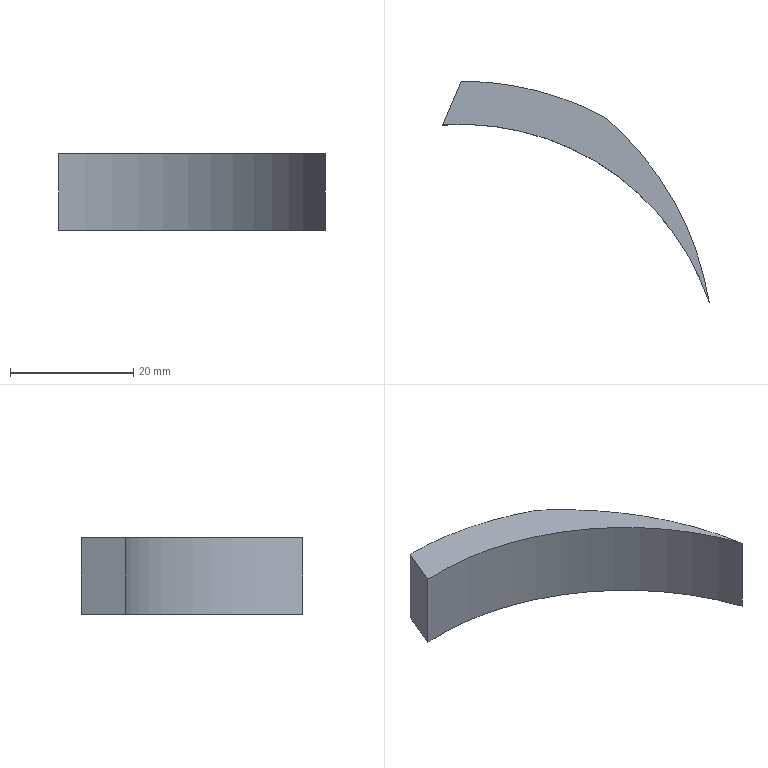Part | SolidWorks | features BaseBody 1 | 1 solid | 6 faces | box 43.285 x 35.96 x 12.5 mm | volume 3482 mm3 | cylinder 3 | plane 3 | commonest cylinder face diameters 85 x1 99 x1 100 x1
STEP:
#1=CARTESIAN_POINT('',(40.285,13.54,6.25));
#2=VERTEX_POINT('',#1);
#3=CARTESIAN_POINT('',(40.285,13.54,-6.25));
#4=VERTEX_POINT('',#3);
#5=CARTESIAN_POINT('',(40.285,13.54,6.25));
#6=DIRECTION('',(0.,0.,-1.));
#7=VECTOR('',#6,1000.);
#8=LINE('',#5,#7);
#9=EDGE_CURVE('',#2,#4,#8,.T.);
#10=ORIENTED_EDGE('',*,*,#9,.F.);
#11=CARTESIAN_POINT('',(-3.,42.394,6.25));
#12=VERTEX_POINT('',#11);
#13=CARTESIAN_POINT('',(0.,0.,6.25));
#14=DIRECTION('',(0.,0.,-1.));
#15=DIRECTION('',(-1.,0.,0.));
#16=AXIS2_PLACEMENT_3D('',#13,#14,#15);
#17=CIRCLE('',#16,42.5);
#18=EDGE_CURVE('',#12,#2,#17,.T.);
#19=ORIENTED_EDGE('',*,*,#18,.F.);
#20=CARTESIAN_POINT('',(-3.,42.394,-6.25));
#21=VERTEX_POINT('',#20);
#22=CARTESIAN_POINT('',(-3.,42.394,6.25));
#23=DIRECTION('',(0.,0.,1.));
#24=VECTOR('',#23,1000.);
#25=LINE('',#22,#24);
#26=EDGE_CURVE('',#21,#12,#25,.T.);
#27=ORIENTED_EDGE('',*,*,#26,.F.);
#28=CARTESIAN_POINT('',(0.,0.,-6.25));
#29=DIRECTION('',(0.,0.,1.));
#30=DIRECTION('',(-1.,0.,0.));
#31=AXIS2_PLACEMENT_3D('',#28,#29,#30);
#32=CIRCLE('',#31,42.5);
#33=EDGE_CURVE('',#4,#21,#32,.T.);
#34=ORIENTED_EDGE('',*,*,#33,.F.);
#35=EDGE_LOOP('',(#10,#19,#27,#34));
#36=FACE_OUTER_BOUND('',#35,.T.);
#37=CARTESIAN_POINT('',(0.,0.,6.25));
#38=DIRECTION('',(0.,0.,-1.));
#39=DIRECTION('',(-1.,0.,0.));
#40=AXIS2_PLACEMENT_3D('',#37,#38,#39);
#41=CYLINDRICAL_SURFACE('',#40,42.5);
#42=ADVANCED_FACE('',(#36),#41,.F.);
#43=CARTESIAN_POINT('',(23.284,43.682,-6.25));
#44=VERTEX_POINT('',#43);
#45=CARTESIAN_POINT('',(-9.074,5.565,-6.25));
#46=DIRECTION('',(0.,0.,1.));
#47=DIRECTION('',(-1.,0.,0.));
#48=AXIS2_PLACEMENT_3D('',#45,#46,#47);
#49=CIRCLE('',#48,50.);
#50=EDGE_CURVE('',#4,#44,#49,.T.);
#51=ORIENTED_EDGE('',*,*,#50,.F.);
#52=ORIENTED_EDGE('',*,*,#33,.T.);
#53=CARTESIAN_POINT('',(0.,49.5,-6.25));
#54=VERTEX_POINT('',#53);
#55=CARTESIAN_POINT('',(0.,49.5,-6.25));
#56=DIRECTION('',(-0.3889,-0.9213,0.));
#57=VECTOR('',#56,1000.);
#58=LINE('',#55,#57);
#59=EDGE_CURVE('',#54,#21,#58,.T.);
#60=ORIENTED_EDGE('',*,*,#59,.F.);
#61=CARTESIAN_POINT('',(0.,0.,-6.25));
#62=DIRECTION('',(0.,0.,1.));
#63=DIRECTION('',(-1.,0.,0.));
#64=AXIS2_PLACEMENT_3D('',#61,#62,#63);
#65=CIRCLE('',#64,49.5);
#66=EDGE_CURVE('',#44,#54,#65,.T.);
#67=ORIENTED_EDGE('',*,*,#66,.F.);
#68=EDGE_LOOP('',(#51,#52,#60,#67));
#69=FACE_OUTER_BOUND('',#68,.T.);
#70=CARTESIAN_POINT('',(0.,0.,-6.25));
#71=DIRECTION('',(0.,0.,1.));
#72=DIRECTION('',(1.,0.,0.));
#73=AXIS2_PLACEMENT_3D('',#70,#71,#72);
#74=PLANE('',#73);
#75=ADVANCED_FACE('',(#69),#74,.F.);
#76=CARTESIAN_POINT('',(23.284,43.682,6.25));
#77=VERTEX_POINT('',#76);
#78=CARTESIAN_POINT('',(-9.074,5.565,6.25));
#79=DIRECTION('',(0.,0.,-1.));
#80=DIRECTION('',(-1.,0.,0.));
#81=AXIS2_PLACEMENT_3D('',#78,#79,#80);
#82=CIRCLE('',#81,50.);
#83=EDGE_CURVE('',#77,#2,#82,.T.);
#84=ORIENTED_EDGE('',*,*,#83,.T.);
#85=ORIENTED_EDGE('',*,*,#9,.T.);
#86=ORIENTED_EDGE('',*,*,#50,.T.);
#87=CARTESIAN_POINT('',(23.284,43.682,6.25));
#88=DIRECTION('',(0.,0.,1.));
#89=VECTOR('',#88,1000.);
#90=LINE('',#87,#89);
#91=EDGE_CURVE('',#44,#77,#90,.T.);
#92=ORIENTED_EDGE('',*,*,#91,.T.);
#93=EDGE_LOOP('',(#84,#85,#86,#92));
#94=FACE_OUTER_BOUND('',#93,.T.);
#95=CARTESIAN_POINT('',(-9.074,5.565,6.25));
#96=DIRECTION('',(0.,0.,-1.));
#97=DIRECTION('',(-1.,0.,0.));
#98=AXIS2_PLACEMENT_3D('',#95,#96,#97);
#99=CYLINDRICAL_SURFACE('',#98,50.);
#100=ADVANCED_FACE('',(#94),#99,.T.);
#101=ORIENTED_EDGE('',*,*,#18,.T.);
#102=ORIENTED_EDGE('',*,*,#83,.F.);
#103=CARTESIAN_POINT('',(0.,49.5,6.25));
#104=VERTEX_POINT('',#103);
#105=CARTESIAN_POINT('',(0.,0.,6.25));
#106=DIRECTION('',(0.,0.,1.));
#107=DIRECTION('',(-1.,0.,0.));
#108=AXIS2_PLACEMENT_3D('',#105,#106,#107);
#109=CIRCLE('',#108,49.5);
#110=EDGE_CURVE('',#77,#104,#109,.T.);
#111=ORIENTED_EDGE('',*,*,#110,.T.);
#112=CARTESIAN_POINT('',(0.,49.5,6.25));
#113=DIRECTION('',(-0.3889,-0.9213,0.));
#114=VECTOR('',#113,1000.);
#115=LINE('',#112,#114);
#116=EDGE_CURVE('',#104,#12,#115,.T.);
#117=ORIENTED_EDGE('',*,*,#116,.T.);
#118=EDGE_LOOP('',(#101,#102,#111,#117));
#119=FACE_OUTER_BOUND('',#118,.T.);
#120=CARTESIAN_POINT('',(0.,0.,6.25));
#121=DIRECTION('',(0.,0.,1.));
#122=DIRECTION('',(1.,0.,0.));
#123=AXIS2_PLACEMENT_3D('',#120,#121,#122);
#124=PLANE('',#123);
#125=ADVANCED_FACE('',(#119),#124,.T.);
#126=ORIENTED_EDGE('',*,*,#26,.T.);
#127=ORIENTED_EDGE('',*,*,#116,.F.);
#128=CARTESIAN_POINT('',(0.,49.5,6.25));
#129=DIRECTION('',(0.,0.,1.));
#130=VECTOR('',#129,1000.);
#131=LINE('',#128,#130);
#132=EDGE_CURVE('',#54,#104,#131,.T.);
#133=ORIENTED_EDGE('',*,*,#132,.F.);
#134=ORIENTED_EDGE('',*,*,#59,.T.);
#135=EDGE_LOOP('',(#126,#127,#133,#134));
#136=FACE_OUTER_BOUND('',#135,.T.);
#137=CARTESIAN_POINT('',(0.,49.5,6.25));
#138=DIRECTION('',(0.9213,-0.3889,0.));
#139=DIRECTION('',(0.3889,0.9213,0.));
#140=AXIS2_PLACEMENT_3D('',#137,#138,#139);
#141=PLANE('',#140);
#142=ADVANCED_FACE('',(#136),#141,.F.);
#143=ORIENTED_EDGE('',*,*,#110,.F.);
#144=ORIENTED_EDGE('',*,*,#91,.F.);
#145=ORIENTED_EDGE('',*,*,#66,.T.);
#146=ORIENTED_EDGE('',*,*,#132,.T.);
#147=EDGE_LOOP('',(#143,#144,#145,#146));
#148=FACE_OUTER_BOUND('',#147,.T.);
#149=CARTESIAN_POINT('',(0.,0.,6.25));
#150=DIRECTION('',(0.,0.,-1.));
#151=DIRECTION('',(-1.,0.,0.));
#152=AXIS2_PLACEMENT_3D('',#149,#150,#151);
#153=CYLINDRICAL_SURFACE('',#152,49.5);
#154=ADVANCED_FACE('',(#148),#153,.T.);
#155=CLOSED_SHELL('',(#42,#75,#100,#125,#142,#154));
#156=MANIFOLD_SOLID_BREP('',#155);
#157=CARTESIAN_POINT('',(0.,0.,0.));
#158=DIRECTION('',(0.,0.,1.));
#159=DIRECTION('',(1.,0.,0.));
#160=AXIS2_PLACEMENT_3D('',#157,#158,#159);
#161=(LENGTH_UNIT()NAMED_UNIT(*)SI_UNIT(.MILLI.,.METRE.));
#162=UNCERTAINTY_MEASURE_WITH_UNIT(LENGTH_MEASURE(0.00001),#161,'','');
#163=(NAMED_UNIT(*)PLANE_ANGLE_UNIT()SI_UNIT($,.RADIAN.));
#164=(NAMED_UNIT(*)SI_UNIT($,.STERADIAN.)SOLID_ANGLE_UNIT());
#165=(GEOMETRIC_REPRESENTATION_CONTEXT(3)GLOBAL_UNCERTAINTY_ASSIGNED_CONTEXT((#162))GLOBAL_UNIT_ASSIGNED_CONTEXT((#161,#163,#164))REPRESENTATION_CONTEXT('',''));
#166=ADVANCED_BREP_SHAPE_REPRESENTATION('',(#156,#160),#165);